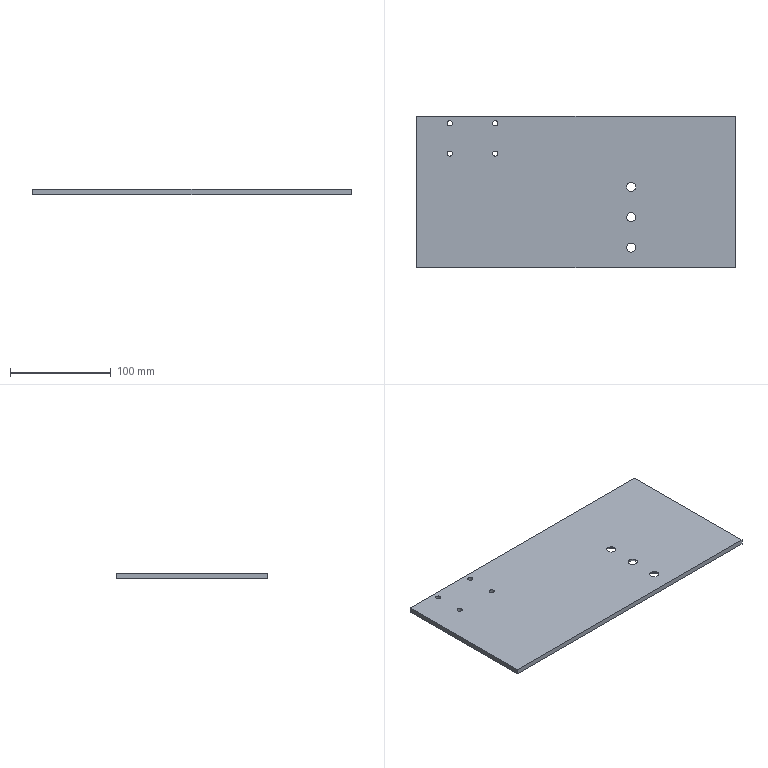Part | NX | features BREP 1 | 1 solid | 16 faces | box 315 x 150 x 5 mm | volume 233869 mm3 | cylinder 7 | plane 6 | cone 3 | commonest cylinder face diameters 5 x4 9 x3
STEP:
#1=CARTESIAN_POINT('',(-77.5,38.,5.));
#2=VERTEX_POINT('',#1);
#3=CARTESIAN_POINT('',(-80.,38.,5.));
#4=DIRECTION('',(0.,0.,1.));
#5=DIRECTION('',(1.,0.,0.));
#6=AXIS2_PLACEMENT_3D('',#3,#4,#5);
#7=CIRCLE('',#6,2.5);
#8=EDGE_CURVE('',#2,#2,#7,.T.);
#9=ORIENTED_EDGE('',*,*,#8,.T.);
#10=EDGE_LOOP('',(#9));
#11=FACE_BOUND('',#10,.T.);
#12=CARTESIAN_POINT('',(-82.5,38.,0.));
#13=VERTEX_POINT('',#12);
#14=CARTESIAN_POINT('',(-80.,38.,0.));
#15=DIRECTION('',(0.,0.,-1.));
#16=DIRECTION('',(-1.,0.,0.));
#17=AXIS2_PLACEMENT_3D('',#14,#15,#16);
#18=CIRCLE('',#17,2.5);
#19=EDGE_CURVE('',#13,#13,#18,.T.);
#20=ORIENTED_EDGE('',*,*,#19,.T.);
#21=EDGE_LOOP('',(#20));
#22=FACE_BOUND('',#21,.T.);
#23=CARTESIAN_POINT('',(-80.,38.,5.));
#24=DIRECTION('',(0.,0.,1.));
#25=DIRECTION('',(1.,0.,0.));
#26=AXIS2_PLACEMENT_3D('',#23,#24,#25);
#27=CYLINDRICAL_SURFACE('',#26,2.5);
#28=ADVANCED_FACE('',(#11,#22),#27,.F.);
#29=CARTESIAN_POINT('',(-122.5,38.,5.));
#30=VERTEX_POINT('',#29);
#31=CARTESIAN_POINT('',(-125.,38.,5.));
#32=DIRECTION('',(0.,0.,1.));
#33=DIRECTION('',(1.,0.,0.));
#34=AXIS2_PLACEMENT_3D('',#31,#32,#33);
#35=CIRCLE('',#34,2.5);
#36=EDGE_CURVE('',#30,#30,#35,.T.);
#37=ORIENTED_EDGE('',*,*,#36,.T.);
#38=EDGE_LOOP('',(#37));
#39=FACE_BOUND('',#38,.T.);
#40=CARTESIAN_POINT('',(-127.5,38.,0.));
#41=VERTEX_POINT('',#40);
#42=CARTESIAN_POINT('',(-125.,38.,0.));
#43=DIRECTION('',(0.,0.,-1.));
#44=DIRECTION('',(-1.,0.,0.));
#45=AXIS2_PLACEMENT_3D('',#42,#43,#44);
#46=CIRCLE('',#45,2.5);
#47=EDGE_CURVE('',#41,#41,#46,.T.);
#48=ORIENTED_EDGE('',*,*,#47,.T.);
#49=EDGE_LOOP('',(#48));
#50=FACE_BOUND('',#49,.T.);
#51=CARTESIAN_POINT('',(-125.,38.,5.));
#52=DIRECTION('',(0.,0.,1.));
#53=DIRECTION('',(1.,0.,0.));
#54=AXIS2_PLACEMENT_3D('',#51,#52,#53);
#55=CYLINDRICAL_SURFACE('',#54,2.5);
#56=ADVANCED_FACE('',(#39,#50),#55,.F.);
#57=CARTESIAN_POINT('',(-122.5,68.,5.));
#58=VERTEX_POINT('',#57);
#59=CARTESIAN_POINT('',(-125.,68.,5.));
#60=DIRECTION('',(0.,0.,1.));
#61=DIRECTION('',(1.,0.,0.));
#62=AXIS2_PLACEMENT_3D('',#59,#60,#61);
#63=CIRCLE('',#62,2.5);
#64=EDGE_CURVE('',#58,#58,#63,.T.);
#65=ORIENTED_EDGE('',*,*,#64,.T.);
#66=EDGE_LOOP('',(#65));
#67=FACE_BOUND('',#66,.T.);
#68=CARTESIAN_POINT('',(-127.5,68.,0.));
#69=VERTEX_POINT('',#68);
#70=CARTESIAN_POINT('',(-125.,68.,0.));
#71=DIRECTION('',(0.,0.,-1.));
#72=DIRECTION('',(-1.,0.,0.));
#73=AXIS2_PLACEMENT_3D('',#70,#71,#72);
#74=CIRCLE('',#73,2.5);
#75=EDGE_CURVE('',#69,#69,#74,.T.);
#76=ORIENTED_EDGE('',*,*,#75,.T.);
#77=EDGE_LOOP('',(#76));
#78=FACE_BOUND('',#77,.T.);
#79=CARTESIAN_POINT('',(-125.,68.,5.));
#80=DIRECTION('',(0.,0.,1.));
#81=DIRECTION('',(1.,0.,0.));
#82=AXIS2_PLACEMENT_3D('',#79,#80,#81);
#83=CYLINDRICAL_SURFACE('',#82,2.5);
#84=ADVANCED_FACE('',(#67,#78),#83,.F.);
#85=CARTESIAN_POINT('',(-77.5,68.,5.));
#86=VERTEX_POINT('',#85);
#87=CARTESIAN_POINT('',(-80.,68.,5.));
#88=DIRECTION('',(0.,0.,1.));
#89=DIRECTION('',(1.,0.,0.));
#90=AXIS2_PLACEMENT_3D('',#87,#88,#89);
#91=CIRCLE('',#90,2.5);
#92=EDGE_CURVE('',#86,#86,#91,.T.);
#93=ORIENTED_EDGE('',*,*,#92,.T.);
#94=EDGE_LOOP('',(#93));
#95=FACE_BOUND('',#94,.T.);
#96=CARTESIAN_POINT('',(-82.5,68.,0.));
#97=VERTEX_POINT('',#96);
#98=CARTESIAN_POINT('',(-80.,68.,0.));
#99=DIRECTION('',(0.,0.,-1.));
#100=DIRECTION('',(-1.,0.,0.));
#101=AXIS2_PLACEMENT_3D('',#98,#99,#100);
#102=CIRCLE('',#101,2.5);
#103=EDGE_CURVE('',#97,#97,#102,.T.);
#104=ORIENTED_EDGE('',*,*,#103,.T.);
#105=EDGE_LOOP('',(#104));
#106=FACE_BOUND('',#105,.T.);
#107=CARTESIAN_POINT('',(-80.,68.,5.));
#108=DIRECTION('',(0.,0.,1.));
#109=DIRECTION('',(1.,0.,0.));
#110=AXIS2_PLACEMENT_3D('',#107,#108,#109);
#111=CYLINDRICAL_SURFACE('',#110,2.5);
#112=ADVANCED_FACE('',(#95,#106),#111,.F.);
#113=CARTESIAN_POINT('',(45.7,-55.,0.));
#114=VERTEX_POINT('',#113);
#115=CARTESIAN_POINT('',(54.5,-55.,0.));
#116=DIRECTION('',(0.,0.,-1.));
#117=DIRECTION('',(-1.,0.,0.));
#118=AXIS2_PLACEMENT_3D('',#115,#116,#117);
#119=CIRCLE('',#118,8.8);
#120=EDGE_CURVE('',#114,#114,#119,.T.);
#121=ORIENTED_EDGE('',*,*,#120,.T.);
#122=EDGE_LOOP('',(#121));
#123=FACE_BOUND('',#122,.T.);
#124=CARTESIAN_POINT('',(50.,-55.,4.3));
#125=VERTEX_POINT('',#124);
#126=CARTESIAN_POINT('',(54.5,-55.,4.3));
#127=DIRECTION('',(0.,0.,-1.));
#128=DIRECTION('',(-1.,0.,0.));
#129=AXIS2_PLACEMENT_3D('',#126,#127,#128);
#130=CIRCLE('',#129,4.5);
#131=EDGE_CURVE('',#125,#125,#130,.T.);
#132=ORIENTED_EDGE('',*,*,#131,.F.);
#133=EDGE_LOOP('',(#132));
#134=FACE_BOUND('',#133,.T.);
#135=CARTESIAN_POINT('',(54.5,-55.,0.));
#136=DIRECTION('',(0.,0.,-1.));
#137=DIRECTION('',(-1.,0.,0.));
#138=AXIS2_PLACEMENT_3D('',#135,#136,#137);
#139=CONICAL_SURFACE('',#138,8.8,0.7854);
#140=ADVANCED_FACE('',(#123,#134),#139,.F.);
#141=ORIENTED_EDGE('',*,*,#131,.T.);
#142=EDGE_LOOP('',(#141));
#143=FACE_BOUND('',#142,.T.);
#144=CARTESIAN_POINT('',(50.,-55.,5.));
#145=VERTEX_POINT('',#144);
#146=CARTESIAN_POINT('',(54.5,-55.,5.));
#147=DIRECTION('',(0.,0.,-1.));
#148=DIRECTION('',(-1.,0.,0.));
#149=AXIS2_PLACEMENT_3D('',#146,#147,#148);
#150=CIRCLE('',#149,4.5);
#151=EDGE_CURVE('',#145,#145,#150,.T.);
#152=ORIENTED_EDGE('',*,*,#151,.F.);
#153=EDGE_LOOP('',(#152));
#154=FACE_BOUND('',#153,.T.);
#155=CARTESIAN_POINT('',(54.5,-55.,0.));
#156=DIRECTION('',(0.,0.,-1.));
#157=DIRECTION('',(-1.,0.,0.));
#158=AXIS2_PLACEMENT_3D('',#155,#156,#157);
#159=CYLINDRICAL_SURFACE('',#158,4.5);
#160=ADVANCED_FACE('',(#143,#154),#159,.F.);
#161=CARTESIAN_POINT('',(45.7,-25.,0.));
#162=VERTEX_POINT('',#161);
#163=CARTESIAN_POINT('',(54.5,-25.,0.));
#164=DIRECTION('',(0.,0.,-1.));
#165=DIRECTION('',(-1.,0.,0.));
#166=AXIS2_PLACEMENT_3D('',#163,#164,#165);
#167=CIRCLE('',#166,8.8);
#168=EDGE_CURVE('',#162,#162,#167,.T.);
#169=ORIENTED_EDGE('',*,*,#168,.T.);
#170=EDGE_LOOP('',(#169));
#171=FACE_BOUND('',#170,.T.);
#172=CARTESIAN_POINT('',(50.,-25.,4.3));
#173=VERTEX_POINT('',#172);
#174=CARTESIAN_POINT('',(54.5,-25.,4.3));
#175=DIRECTION('',(0.,0.,-1.));
#176=DIRECTION('',(-1.,0.,0.));
#177=AXIS2_PLACEMENT_3D('',#174,#175,#176);
#178=CIRCLE('',#177,4.5);
#179=EDGE_CURVE('',#173,#173,#178,.T.);
#180=ORIENTED_EDGE('',*,*,#179,.F.);
#181=EDGE_LOOP('',(#180));
#182=FACE_BOUND('',#181,.T.);
#183=CARTESIAN_POINT('',(54.5,-25.,0.));
#184=DIRECTION('',(0.,0.,-1.));
#185=DIRECTION('',(-1.,0.,0.));
#186=AXIS2_PLACEMENT_3D('',#183,#184,#185);
#187=CONICAL_SURFACE('',#186,8.8,0.7854);
#188=ADVANCED_FACE('',(#171,#182),#187,.F.);
#189=ORIENTED_EDGE('',*,*,#179,.T.);
#190=EDGE_LOOP('',(#189));
#191=FACE_BOUND('',#190,.T.);
#192=CARTESIAN_POINT('',(50.,-25.,5.));
#193=VERTEX_POINT('',#192);
#194=CARTESIAN_POINT('',(54.5,-25.,5.));
#195=DIRECTION('',(0.,0.,-1.));
#196=DIRECTION('',(-1.,0.,0.));
#197=AXIS2_PLACEMENT_3D('',#194,#195,#196);
#198=CIRCLE('',#197,4.5);
#199=EDGE_CURVE('',#193,#193,#198,.T.);
#200=ORIENTED_EDGE('',*,*,#199,.F.);
#201=EDGE_LOOP('',(#200));
#202=FACE_BOUND('',#201,.T.);
#203=CARTESIAN_POINT('',(54.5,-25.,0.));
#204=DIRECTION('',(0.,0.,-1.));
#205=DIRECTION('',(-1.,0.,0.));
#206=AXIS2_PLACEMENT_3D('',#203,#204,#205);
#207=CYLINDRICAL_SURFACE('',#206,4.5);
#208=ADVANCED_FACE('',(#191,#202),#207,.F.);
#209=CARTESIAN_POINT('',(45.7,5.,0.));
#210=VERTEX_POINT('',#209);
#211=CARTESIAN_POINT('',(54.5,5.,0.));
#212=DIRECTION('',(0.,0.,-1.));
#213=DIRECTION('',(-1.,0.,0.));
#214=AXIS2_PLACEMENT_3D('',#211,#212,#213);
#215=CIRCLE('',#214,8.8);
#216=EDGE_CURVE('',#210,#210,#215,.T.);
#217=ORIENTED_EDGE('',*,*,#216,.T.);
#218=EDGE_LOOP('',(#217));
#219=FACE_BOUND('',#218,.T.);
#220=CARTESIAN_POINT('',(50.,5.,4.3));
#221=VERTEX_POINT('',#220);
#222=CARTESIAN_POINT('',(54.5,5.,4.3));
#223=DIRECTION('',(0.,0.,-1.));
#224=DIRECTION('',(-1.,0.,0.));
#225=AXIS2_PLACEMENT_3D('',#222,#223,#224);
#226=CIRCLE('',#225,4.5);
#227=EDGE_CURVE('',#221,#221,#226,.T.);
#228=ORIENTED_EDGE('',*,*,#227,.F.);
#229=EDGE_LOOP('',(#228));
#230=FACE_BOUND('',#229,.T.);
#231=CARTESIAN_POINT('',(54.5,5.,0.));
#232=DIRECTION('',(0.,0.,-1.));
#233=DIRECTION('',(-1.,0.,0.));
#234=AXIS2_PLACEMENT_3D('',#231,#232,#233);
#235=CONICAL_SURFACE('',#234,8.8,0.7854);
#236=ADVANCED_FACE('',(#219,#230),#235,.F.);
#237=ORIENTED_EDGE('',*,*,#227,.T.);
#238=EDGE_LOOP('',(#237));
#239=FACE_BOUND('',#238,.T.);
#240=CARTESIAN_POINT('',(50.,5.,5.));
#241=VERTEX_POINT('',#240);
#242=CARTESIAN_POINT('',(54.5,5.,5.));
#243=DIRECTION('',(0.,0.,-1.));
#244=DIRECTION('',(-1.,0.,0.));
#245=AXIS2_PLACEMENT_3D('',#242,#243,#244);
#246=CIRCLE('',#245,4.5);
#247=EDGE_CURVE('',#241,#241,#246,.T.);
#248=ORIENTED_EDGE('',*,*,#247,.F.);
#249=EDGE_LOOP('',(#248));
#250=FACE_BOUND('',#249,.T.);
#251=CARTESIAN_POINT('',(54.5,5.,0.));
#252=DIRECTION('',(0.,0.,-1.));
#253=DIRECTION('',(-1.,0.,0.));
#254=AXIS2_PLACEMENT_3D('',#251,#252,#253);
#255=CYLINDRICAL_SURFACE('',#254,4.5);
#256=ADVANCED_FACE('',(#239,#250),#255,.F.);
#257=ORIENTED_EDGE('',*,*,#36,.F.);
#258=EDGE_LOOP('',(#257));
#259=FACE_BOUND('',#258,.T.);
#260=ORIENTED_EDGE('',*,*,#64,.F.);
#261=EDGE_LOOP('',(#260));
#262=FACE_BOUND('',#261,.T.);
#263=ORIENTED_EDGE('',*,*,#92,.F.);
#264=EDGE_LOOP('',(#263));
#265=FACE_BOUND('',#264,.T.);
#266=ORIENTED_EDGE('',*,*,#151,.T.);
#267=EDGE_LOOP('',(#266));
#268=FACE_BOUND('',#267,.T.);
#269=ORIENTED_EDGE('',*,*,#199,.T.);
#270=EDGE_LOOP('',(#269));
#271=FACE_BOUND('',#270,.T.);
#272=ORIENTED_EDGE('',*,*,#247,.T.);
#273=EDGE_LOOP('',(#272));
#274=FACE_BOUND('',#273,.T.);
#275=CARTESIAN_POINT('',(157.5,-75.,5.));
#276=VERTEX_POINT('',#275);
#277=CARTESIAN_POINT('',(157.5,75.,5.));
#278=VERTEX_POINT('',#277);
#279=CARTESIAN_POINT('',(157.5,-75.,5.));
#280=DIRECTION('',(0.,1.,0.));
#281=VECTOR('',#280,1000.);
#282=LINE('',#279,#281);
#283=EDGE_CURVE('',#276,#278,#282,.T.);
#284=ORIENTED_EDGE('',*,*,#283,.T.);
#285=CARTESIAN_POINT('',(-157.5,75.,5.));
#286=VERTEX_POINT('',#285);
#287=CARTESIAN_POINT('',(-157.5,75.,5.));
#288=DIRECTION('',(-1.,0.,0.));
#289=VECTOR('',#288,1000.);
#290=LINE('',#287,#289);
#291=EDGE_CURVE('',#278,#286,#290,.T.);
#292=ORIENTED_EDGE('',*,*,#291,.T.);
#293=CARTESIAN_POINT('',(-157.5,-75.,5.));
#294=VERTEX_POINT('',#293);
#295=CARTESIAN_POINT('',(-157.5,-75.,5.));
#296=DIRECTION('',(0.,-1.,0.));
#297=VECTOR('',#296,1000.);
#298=LINE('',#295,#297);
#299=EDGE_CURVE('',#286,#294,#298,.T.);
#300=ORIENTED_EDGE('',*,*,#299,.T.);
#301=CARTESIAN_POINT('',(-157.5,-75.,5.));
#302=DIRECTION('',(1.,0.,0.));
#303=VECTOR('',#302,1000.);
#304=LINE('',#301,#303);
#305=EDGE_CURVE('',#294,#276,#304,.T.);
#306=ORIENTED_EDGE('',*,*,#305,.T.);
#307=EDGE_LOOP('',(#284,#292,#300,#306));
#308=FACE_BOUND('',#307,.T.);
#309=ORIENTED_EDGE('',*,*,#8,.F.);
#310=EDGE_LOOP('',(#309));
#311=FACE_BOUND('',#310,.T.);
#312=CARTESIAN_POINT('',(0.,0.,5.));
#313=DIRECTION('',(0.,0.,-1.));
#314=DIRECTION('',(-1.,0.,0.));
#315=AXIS2_PLACEMENT_3D('',#312,#313,#314);
#316=PLANE('',#315);
#317=ADVANCED_FACE('',(#259,#262,#265,#268,#271,#274,#308,#311),#316,.F.);
#318=CARTESIAN_POINT('',(157.5,-75.,0.));
#319=VERTEX_POINT('',#318);
#320=CARTESIAN_POINT('',(157.5,75.,0.));
#321=VERTEX_POINT('',#320);
#322=CARTESIAN_POINT('',(157.5,-75.,0.));
#323=DIRECTION('',(0.,1.,0.));
#324=VECTOR('',#323,1000.);
#325=LINE('',#322,#324);
#326=EDGE_CURVE('',#319,#321,#325,.T.);
#327=ORIENTED_EDGE('',*,*,#326,.T.);
#328=CARTESIAN_POINT('',(157.5,75.,5.));
#329=DIRECTION('',(0.,0.,-1.));
#330=VECTOR('',#329,1000.);
#331=LINE('',#328,#330);
#332=EDGE_CURVE('',#278,#321,#331,.T.);
#333=ORIENTED_EDGE('',*,*,#332,.F.);
#334=ORIENTED_EDGE('',*,*,#283,.F.);
#335=CARTESIAN_POINT('',(157.5,-75.,5.));
#336=DIRECTION('',(0.,0.,-1.));
#337=VECTOR('',#336,1000.);
#338=LINE('',#335,#337);
#339=EDGE_CURVE('',#276,#319,#338,.T.);
#340=ORIENTED_EDGE('',*,*,#339,.T.);
#341=EDGE_LOOP('',(#327,#333,#334,#340));
#342=FACE_BOUND('',#341,.T.);
#343=CARTESIAN_POINT('',(157.5,-75.,5.));
#344=DIRECTION('',(-1.,0.,0.));
#345=DIRECTION('',(0.,0.,1.));
#346=AXIS2_PLACEMENT_3D('',#343,#344,#345);
#347=PLANE('',#346);
#348=ADVANCED_FACE('',(#342),#347,.F.);
#349=CARTESIAN_POINT('',(-157.5,75.,0.));
#350=VERTEX_POINT('',#349);
#351=CARTESIAN_POINT('',(-157.5,75.,0.));
#352=DIRECTION('',(-1.,0.,0.));
#353=VECTOR('',#352,1000.);
#354=LINE('',#351,#353);
#355=EDGE_CURVE('',#321,#350,#354,.T.);
#356=ORIENTED_EDGE('',*,*,#355,.T.);
#357=CARTESIAN_POINT('',(-157.5,75.,5.));
#358=DIRECTION('',(0.,0.,-1.));
#359=VECTOR('',#358,1000.);
#360=LINE('',#357,#359);
#361=EDGE_CURVE('',#286,#350,#360,.T.);
#362=ORIENTED_EDGE('',*,*,#361,.F.);
#363=ORIENTED_EDGE('',*,*,#291,.F.);
#364=ORIENTED_EDGE('',*,*,#332,.T.);
#365=EDGE_LOOP('',(#356,#362,#363,#364));
#366=FACE_BOUND('',#365,.T.);
#367=CARTESIAN_POINT('',(-157.5,75.,5.));
#368=DIRECTION('',(0.,-1.,0.));
#369=DIRECTION('',(0.,0.,-1.));
#370=AXIS2_PLACEMENT_3D('',#367,#368,#369);
#371=PLANE('',#370);
#372=ADVANCED_FACE('',(#366),#371,.F.);
#373=CARTESIAN_POINT('',(-157.5,-75.,0.));
#374=VERTEX_POINT('',#373);
#375=CARTESIAN_POINT('',(-157.5,-75.,0.));
#376=DIRECTION('',(0.,-1.,0.));
#377=VECTOR('',#376,1000.);
#378=LINE('',#375,#377);
#379=EDGE_CURVE('',#350,#374,#378,.T.);
#380=ORIENTED_EDGE('',*,*,#379,.T.);
#381=CARTESIAN_POINT('',(-157.5,-75.,5.));
#382=DIRECTION('',(0.,0.,-1.));
#383=VECTOR('',#382,1000.);
#384=LINE('',#381,#383);
#385=EDGE_CURVE('',#294,#374,#384,.T.);
#386=ORIENTED_EDGE('',*,*,#385,.F.);
#387=ORIENTED_EDGE('',*,*,#299,.F.);
#388=ORIENTED_EDGE('',*,*,#361,.T.);
#389=EDGE_LOOP('',(#380,#386,#387,#388));
#390=FACE_BOUND('',#389,.T.);
#391=CARTESIAN_POINT('',(-157.5,-75.,5.));
#392=DIRECTION('',(1.,0.,0.));
#393=DIRECTION('',(0.,0.,-1.));
#394=AXIS2_PLACEMENT_3D('',#391,#392,#393);
#395=PLANE('',#394);
#396=ADVANCED_FACE('',(#390),#395,.F.);
#397=CARTESIAN_POINT('',(-157.5,-75.,0.));
#398=DIRECTION('',(1.,0.,0.));
#399=VECTOR('',#398,1000.);
#400=LINE('',#397,#399);
#401=EDGE_CURVE('',#374,#319,#400,.T.);
#402=ORIENTED_EDGE('',*,*,#401,.T.);
#403=ORIENTED_EDGE('',*,*,#339,.F.);
#404=ORIENTED_EDGE('',*,*,#305,.F.);
#405=ORIENTED_EDGE('',*,*,#385,.T.);
#406=EDGE_LOOP('',(#402,#403,#404,#405));
#407=FACE_BOUND('',#406,.T.);
#408=CARTESIAN_POINT('',(-157.5,-75.,5.));
#409=DIRECTION('',(0.,1.,0.));
#410=DIRECTION('',(0.,0.,1.));
#411=AXIS2_PLACEMENT_3D('',#408,#409,#410);
#412=PLANE('',#411);
#413=ADVANCED_FACE('',(#407),#412,.F.);
#414=ORIENTED_EDGE('',*,*,#19,.F.);
#415=EDGE_LOOP('',(#414));
#416=FACE_BOUND('',#415,.T.);
#417=ORIENTED_EDGE('',*,*,#47,.F.);
#418=EDGE_LOOP('',(#417));
#419=FACE_BOUND('',#418,.T.);
#420=ORIENTED_EDGE('',*,*,#75,.F.);
#421=EDGE_LOOP('',(#420));
#422=FACE_BOUND('',#421,.T.);
#423=ORIENTED_EDGE('',*,*,#103,.F.);
#424=EDGE_LOOP('',(#423));
#425=FACE_BOUND('',#424,.T.);
#426=ORIENTED_EDGE('',*,*,#120,.F.);
#427=EDGE_LOOP('',(#426));
#428=FACE_BOUND('',#427,.T.);
#429=ORIENTED_EDGE('',*,*,#168,.F.);
#430=EDGE_LOOP('',(#429));
#431=FACE_BOUND('',#430,.T.);
#432=ORIENTED_EDGE('',*,*,#216,.F.);
#433=EDGE_LOOP('',(#432));
#434=FACE_BOUND('',#433,.T.);
#435=ORIENTED_EDGE('',*,*,#326,.F.);
#436=ORIENTED_EDGE('',*,*,#401,.F.);
#437=ORIENTED_EDGE('',*,*,#379,.F.);
#438=ORIENTED_EDGE('',*,*,#355,.F.);
#439=EDGE_LOOP('',(#435,#436,#437,#438));
#440=FACE_BOUND('',#439,.T.);
#441=CARTESIAN_POINT('',(0.,0.,0.));
#442=DIRECTION('',(0.,0.,-1.));
#443=DIRECTION('',(-1.,0.,0.));
#444=AXIS2_PLACEMENT_3D('',#441,#442,#443);
#445=PLANE('',#444);
#446=ADVANCED_FACE('',(#416,#419,#422,#425,#428,#431,#434,#440),#445,.T.);
#447=CLOSED_SHELL('',(#28,#56,#84,#112,#140,#160,#188,#208,#236,#256,#317,#348,#372,#396,#413,#446));
#448=MANIFOLD_SOLID_BREP('',#447);
#449=(LENGTH_UNIT()NAMED_UNIT(*)SI_UNIT(.MILLI.,.METRE.));
#450=UNCERTAINTY_MEASURE_WITH_UNIT(LENGTH_MEASURE(0.00001),#449,'','');
#451=(NAMED_UNIT(*)PLANE_ANGLE_UNIT()SI_UNIT($,.RADIAN.));
#452=(NAMED_UNIT(*)SI_UNIT($,.STERADIAN.)SOLID_ANGLE_UNIT());
#453=(GEOMETRIC_REPRESENTATION_CONTEXT(3)GLOBAL_UNCERTAINTY_ASSIGNED_CONTEXT((#450))GLOBAL_UNIT_ASSIGNED_CONTEXT((#449,#451,#452))REPRESENTATION_CONTEXT('',''));
#454=ADVANCED_BREP_SHAPE_REPRESENTATION('',(#448),#453);